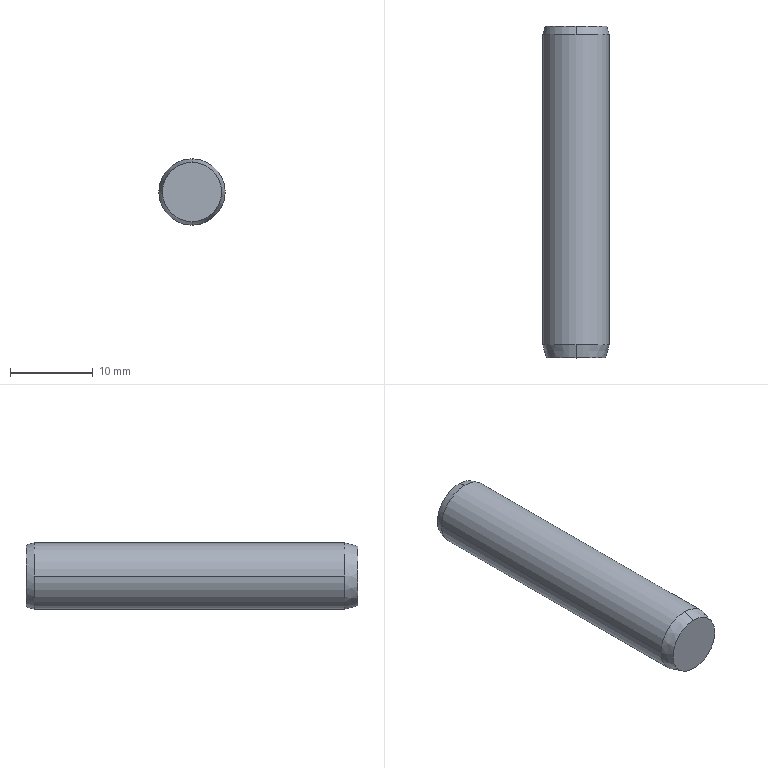Part | STEP file | 1 solid | 16 faces | box 8 x 40 x 8 mm | volume 1821 mm3 | cone 8 | cylinder 6 | plane 2 | commonest cylinder face diameters 4.134 x2 5.3 x2 8 x2
STEP:
#1=CARTESIAN_POINT('',(0.,-40.,3.571));
#2=VERTEX_POINT('',#1);
#3=CARTESIAN_POINT('',(0.,-40.,-3.571));
#4=VERTEX_POINT('',#3);
#5=CARTESIAN_POINT('',(0.,-40.,0.));
#6=DIRECTION('',(0.,1.,0.));
#7=DIRECTION('',(0.,0.,1.));
#8=AXIS2_PLACEMENT_3D('',#5,#6,#7);
#9=CIRCLE('',#8,3.571);
#10=EDGE_CURVE('',#2,#4,#9,.T.);
#11=ORIENTED_EDGE('',*,*,#10,.T.);
#12=CARTESIAN_POINT('',(0.,-38.4,-4.));
#13=VERTEX_POINT('',#12);
#14=CARTESIAN_POINT('',(0.,-40.,-3.571));
#15=DIRECTION('',(0.,0.9659,-0.2588));
#16=VECTOR('',#15,1000.);
#17=LINE('',#14,#16);
#18=EDGE_CURVE('',#4,#13,#17,.T.);
#19=ORIENTED_EDGE('',*,*,#18,.T.);
#20=CARTESIAN_POINT('',(4.,-38.4,0.));
#21=VERTEX_POINT('',#20);
#22=CARTESIAN_POINT('',(0.,-38.4,0.));
#23=DIRECTION('',(0.,1.,0.));
#24=DIRECTION('',(0.,0.,1.));
#25=AXIS2_PLACEMENT_3D('',#22,#23,#24);
#26=CIRCLE('',#25,4.);
#27=EDGE_CURVE('',#21,#13,#26,.T.);
#28=ORIENTED_EDGE('',*,*,#27,.F.);
#29=CARTESIAN_POINT('',(0.,-38.4,4.));
#30=VERTEX_POINT('',#29);
#31=CARTESIAN_POINT('',(0.,-38.4,0.));
#32=DIRECTION('',(0.,1.,0.));
#33=DIRECTION('',(0.,0.,1.));
#34=AXIS2_PLACEMENT_3D('',#31,#32,#33);
#35=CIRCLE('',#34,4.);
#36=EDGE_CURVE('',#30,#21,#35,.T.);
#37=ORIENTED_EDGE('',*,*,#36,.F.);
#38=CARTESIAN_POINT('',(0.,-40.,3.571));
#39=DIRECTION('',(0.,0.9659,0.2588));
#40=VECTOR('',#39,1000.);
#41=LINE('',#38,#40);
#42=EDGE_CURVE('',#2,#30,#41,.T.);
#43=ORIENTED_EDGE('',*,*,#42,.F.);
#44=EDGE_LOOP('',(#11,#19,#28,#37,#43));
#45=FACE_OUTER_BOUND('',#44,.T.);
#46=CARTESIAN_POINT('',(0.,-40.,0.));
#47=DIRECTION('',(0.,1.,0.));
#48=DIRECTION('',(0.,0.,1.));
#49=AXIS2_PLACEMENT_3D('',#46,#47,#48);
#50=CONICAL_SURFACE('',#49,3.571,0.2618);
#51=ADVANCED_FACE('',(#45),#50,.T.);
#52=CARTESIAN_POINT('',(-4.,-38.4,0.));
#53=VERTEX_POINT('',#52);
#54=CARTESIAN_POINT('',(0.,-38.4,0.));
#55=DIRECTION('',(0.,1.,0.));
#56=DIRECTION('',(0.,0.,1.));
#57=AXIS2_PLACEMENT_3D('',#54,#55,#56);
#58=CIRCLE('',#57,4.);
#59=EDGE_CURVE('',#53,#30,#58,.T.);
#60=ORIENTED_EDGE('',*,*,#59,.T.);
#61=ORIENTED_EDGE('',*,*,#36,.T.);
#62=CARTESIAN_POINT('',(4.,-1.,0.));
#63=VERTEX_POINT('',#62);
#64=CARTESIAN_POINT('',(4.,-13.193,0.));
#65=DIRECTION('',(0.,1.,0.));
#66=VECTOR('',#65,1000.);
#67=LINE('',#64,#66);
#68=EDGE_CURVE('',#21,#63,#67,.T.);
#69=ORIENTED_EDGE('',*,*,#68,.T.);
#70=CARTESIAN_POINT('',(0.,-1.,4.));
#71=VERTEX_POINT('',#70);
#72=CARTESIAN_POINT('',(0.,-1.,0.));
#73=DIRECTION('',(0.,1.,0.));
#74=DIRECTION('',(0.,0.,1.));
#75=AXIS2_PLACEMENT_3D('',#72,#73,#74);
#76=CIRCLE('',#75,4.);
#77=EDGE_CURVE('',#71,#63,#76,.T.);
#78=ORIENTED_EDGE('',*,*,#77,.F.);
#79=CARTESIAN_POINT('',(-4.,-1.,0.));
#80=VERTEX_POINT('',#79);
#81=CARTESIAN_POINT('',(0.,-1.,0.));
#82=DIRECTION('',(0.,1.,0.));
#83=DIRECTION('',(0.,0.,1.));
#84=AXIS2_PLACEMENT_3D('',#81,#82,#83);
#85=CIRCLE('',#84,4.);
#86=EDGE_CURVE('',#80,#71,#85,.T.);
#87=ORIENTED_EDGE('',*,*,#86,.F.);
#88=CARTESIAN_POINT('',(-4.,-13.193,0.));
#89=DIRECTION('',(0.,1.,0.));
#90=VECTOR('',#89,1000.);
#91=LINE('',#88,#90);
#92=EDGE_CURVE('',#53,#80,#91,.T.);
#93=ORIENTED_EDGE('',*,*,#92,.F.);
#94=EDGE_LOOP('',(#60,#61,#69,#78,#87,#93));
#95=FACE_OUTER_BOUND('',#94,.T.);
#96=CARTESIAN_POINT('',(0.,-13.193,0.));
#97=DIRECTION('',(0.,1.,0.));
#98=DIRECTION('',(-1.,0.,0.));
#99=AXIS2_PLACEMENT_3D('',#96,#97,#98);
#100=CYLINDRICAL_SURFACE('',#99,4.);
#101=ADVANCED_FACE('',(#95),#100,.T.);
#102=CARTESIAN_POINT('',(0.,0.,3.732));
#103=VERTEX_POINT('',#102);
#104=CARTESIAN_POINT('',(0.,0.,-3.732));
#105=VERTEX_POINT('',#104);
#106=CARTESIAN_POINT('',(0.,0.,0.));
#107=DIRECTION('',(0.,1.,0.));
#108=DIRECTION('',(0.,0.,1.));
#109=AXIS2_PLACEMENT_3D('',#106,#107,#108);
#110=CIRCLE('',#109,3.732);
#111=EDGE_CURVE('',#103,#105,#110,.T.);
#112=ORIENTED_EDGE('',*,*,#111,.F.);
#113=CARTESIAN_POINT('',(0.,-1.,4.));
#114=DIRECTION('',(0.,-0.9659,0.2588));
#115=VECTOR('',#114,1000.);
#116=LINE('',#113,#115);
#117=EDGE_CURVE('',#103,#71,#116,.T.);
#118=ORIENTED_EDGE('',*,*,#117,.T.);
#119=ORIENTED_EDGE('',*,*,#77,.T.);
#120=CARTESIAN_POINT('',(0.,-1.,-4.));
#121=VERTEX_POINT('',#120);
#122=CARTESIAN_POINT('',(0.,-1.,0.));
#123=DIRECTION('',(0.,1.,0.));
#124=DIRECTION('',(0.,0.,1.));
#125=AXIS2_PLACEMENT_3D('',#122,#123,#124);
#126=CIRCLE('',#125,4.);
#127=EDGE_CURVE('',#63,#121,#126,.T.);
#128=ORIENTED_EDGE('',*,*,#127,.T.);
#129=CARTESIAN_POINT('',(0.,-1.,-4.));
#130=DIRECTION('',(0.,-0.9659,-0.2588));
#131=VECTOR('',#130,1000.);
#132=LINE('',#129,#131);
#133=EDGE_CURVE('',#105,#121,#132,.T.);
#134=ORIENTED_EDGE('',*,*,#133,.F.);
#135=EDGE_LOOP('',(#112,#118,#119,#128,#134));
#136=FACE_OUTER_BOUND('',#135,.T.);
#137=CARTESIAN_POINT('',(0.,-1.,0.));
#138=DIRECTION('',(0.,-1.,0.));
#139=DIRECTION('',(0.,0.,-1.));
#140=AXIS2_PLACEMENT_3D('',#137,#138,#139);
#141=CONICAL_SURFACE('',#140,4.,0.2618);
#142=ADVANCED_FACE('',(#136),#141,.T.);
#143=CARTESIAN_POINT('',(0.,-13.193,0.));
#144=VERTEX_POINT('',#143);
#145=CARTESIAN_POINT('',(-2.067,-12.,0.));
#146=VERTEX_POINT('',#145);
#147=CARTESIAN_POINT('',(-2.067,-12.,0.));
#148=DIRECTION('',(-0.866,0.5,0.));
#149=VECTOR('',#148,1000.);
#150=LINE('',#147,#149);
#151=EDGE_CURVE('',#144,#146,#150,.T.);
#152=ORIENTED_EDGE('',*,*,#151,.F.);
#153=CARTESIAN_POINT('',(2.067,-12.,0.));
#154=VERTEX_POINT('',#153);
#155=CARTESIAN_POINT('',(2.067,-12.,0.));
#156=DIRECTION('',(0.866,0.5,0.));
#157=VECTOR('',#156,1000.);
#158=LINE('',#155,#157);
#159=EDGE_CURVE('',#144,#154,#158,.T.);
#160=ORIENTED_EDGE('',*,*,#159,.T.);
#161=CARTESIAN_POINT('',(0.,-12.,0.));
#162=DIRECTION('',(0.,1.,0.));
#163=DIRECTION('',(-1.,0.,0.));
#164=AXIS2_PLACEMENT_3D('',#161,#162,#163);
#165=CIRCLE('',#164,2.067);
#166=EDGE_CURVE('',#154,#146,#165,.T.);
#167=ORIENTED_EDGE('',*,*,#166,.T.);
#168=EDGE_LOOP('',(#152,#160,#167));
#169=FACE_OUTER_BOUND('',#168,.T.);
#170=CARTESIAN_POINT('',(0.,-12.,0.));
#171=DIRECTION('',(0.,1.,0.));
#172=DIRECTION('',(-1.,0.,0.));
#173=AXIS2_PLACEMENT_3D('',#170,#171,#172);
#174=CONICAL_SURFACE('',#173,2.067,1.047);
#175=ADVANCED_FACE('',(#169),#174,.F.);
#176=ORIENTED_EDGE('',*,*,#166,.F.);
#177=CARTESIAN_POINT('',(2.067,-1.537,0.));
#178=VERTEX_POINT('',#177);
#179=CARTESIAN_POINT('',(2.067,-13.193,0.));
#180=DIRECTION('',(0.,1.,0.));
#181=VECTOR('',#180,1000.);
#182=LINE('',#179,#181);
#183=EDGE_CURVE('',#154,#178,#182,.T.);
#184=ORIENTED_EDGE('',*,*,#183,.T.);
#185=CARTESIAN_POINT('',(-2.067,-1.537,0.));
#186=VERTEX_POINT('',#185);
#187=CARTESIAN_POINT('',(0.,-1.537,0.));
#188=DIRECTION('',(0.,1.,0.));
#189=DIRECTION('',(-1.,0.,0.));
#190=AXIS2_PLACEMENT_3D('',#187,#188,#189);
#191=CIRCLE('',#190,2.067);
#192=EDGE_CURVE('',#178,#186,#191,.T.);
#193=ORIENTED_EDGE('',*,*,#192,.T.);
#194=CARTESIAN_POINT('',(-2.067,-13.193,0.));
#195=DIRECTION('',(0.,1.,0.));
#196=VECTOR('',#195,1000.);
#197=LINE('',#194,#196);
#198=EDGE_CURVE('',#146,#186,#197,.T.);
#199=ORIENTED_EDGE('',*,*,#198,.F.);
#200=EDGE_LOOP('',(#176,#184,#193,#199));
#201=FACE_OUTER_BOUND('',#200,.T.);
#202=CARTESIAN_POINT('',(0.,-13.193,0.));
#203=DIRECTION('',(0.,1.,0.));
#204=DIRECTION('',(-1.,0.,0.));
#205=AXIS2_PLACEMENT_3D('',#202,#203,#204);
#206=CYLINDRICAL_SURFACE('',#205,2.067);
#207=ADVANCED_FACE('',(#201),#206,.F.);
#208=ORIENTED_EDGE('',*,*,#192,.F.);
#209=CARTESIAN_POINT('',(2.65,-1.2,0.));
#210=VERTEX_POINT('',#209);
#211=CARTESIAN_POINT('',(2.65,-1.2,0.));
#212=DIRECTION('',(0.866,0.5,0.));
#213=VECTOR('',#212,1000.);
#214=LINE('',#211,#213);
#215=EDGE_CURVE('',#178,#210,#214,.T.);
#216=ORIENTED_EDGE('',*,*,#215,.T.);
#217=CARTESIAN_POINT('',(-2.65,-1.2,0.));
#218=VERTEX_POINT('',#217);
#219=CARTESIAN_POINT('',(0.,-1.2,0.));
#220=DIRECTION('',(0.,1.,0.));
#221=DIRECTION('',(-1.,0.,0.));
#222=AXIS2_PLACEMENT_3D('',#219,#220,#221);
#223=CIRCLE('',#222,2.65);
#224=EDGE_CURVE('',#210,#218,#223,.T.);
#225=ORIENTED_EDGE('',*,*,#224,.T.);
#226=CARTESIAN_POINT('',(-2.65,-1.2,0.));
#227=DIRECTION('',(-0.866,0.5,0.));
#228=VECTOR('',#227,1000.);
#229=LINE('',#226,#228);
#230=EDGE_CURVE('',#186,#218,#229,.T.);
#231=ORIENTED_EDGE('',*,*,#230,.F.);
#232=EDGE_LOOP('',(#208,#216,#225,#231));
#233=FACE_OUTER_BOUND('',#232,.T.);
#234=CARTESIAN_POINT('',(0.,-1.2,0.));
#235=DIRECTION('',(0.,1.,0.));
#236=DIRECTION('',(-1.,0.,0.));
#237=AXIS2_PLACEMENT_3D('',#234,#235,#236);
#238=CONICAL_SURFACE('',#237,2.65,1.047);
#239=ADVANCED_FACE('',(#233),#238,.F.);
#240=ORIENTED_EDGE('',*,*,#224,.F.);
#241=CARTESIAN_POINT('',(2.65,0.,0.));
#242=VERTEX_POINT('',#241);
#243=CARTESIAN_POINT('',(2.65,-13.193,0.));
#244=DIRECTION('',(0.,1.,0.));
#245=VECTOR('',#244,1000.);
#246=LINE('',#243,#245);
#247=EDGE_CURVE('',#210,#242,#246,.T.);
#248=ORIENTED_EDGE('',*,*,#247,.T.);
#249=CARTESIAN_POINT('',(-2.65,0.,0.));
#250=VERTEX_POINT('',#249);
#251=CARTESIAN_POINT('',(0.,0.,0.));
#252=DIRECTION('',(0.,1.,0.));
#253=DIRECTION('',(-1.,0.,0.));
#254=AXIS2_PLACEMENT_3D('',#251,#252,#253);
#255=CIRCLE('',#254,2.65);
#256=EDGE_CURVE('',#242,#250,#255,.T.);
#257=ORIENTED_EDGE('',*,*,#256,.T.);
#258=CARTESIAN_POINT('',(-2.65,-13.193,0.));
#259=DIRECTION('',(0.,1.,0.));
#260=VECTOR('',#259,1000.);
#261=LINE('',#258,#260);
#262=EDGE_CURVE('',#218,#250,#261,.T.);
#263=ORIENTED_EDGE('',*,*,#262,.F.);
#264=EDGE_LOOP('',(#240,#248,#257,#263));
#265=FACE_OUTER_BOUND('',#264,.T.);
#266=CARTESIAN_POINT('',(0.,-13.193,0.));
#267=DIRECTION('',(0.,1.,0.));
#268=DIRECTION('',(-1.,0.,0.));
#269=AXIS2_PLACEMENT_3D('',#266,#267,#268);
#270=CYLINDRICAL_SURFACE('',#269,2.65);
#271=ADVANCED_FACE('',(#265),#270,.F.);
#272=CARTESIAN_POINT('',(0.,0.,0.));
#273=DIRECTION('',(0.,1.,0.));
#274=DIRECTION('',(-1.,0.,0.));
#275=AXIS2_PLACEMENT_3D('',#272,#273,#274);
#276=CIRCLE('',#275,2.65);
#277=EDGE_CURVE('',#250,#242,#276,.T.);
#278=ORIENTED_EDGE('',*,*,#277,.F.);
#279=ORIENTED_EDGE('',*,*,#256,.F.);
#280=EDGE_LOOP('',(#278,#279));
#281=FACE_BOUND('',#280,.T.);
#282=CARTESIAN_POINT('',(0.,0.,0.));
#283=DIRECTION('',(0.,1.,0.));
#284=DIRECTION('',(0.,0.,1.));
#285=AXIS2_PLACEMENT_3D('',#282,#283,#284);
#286=CIRCLE('',#285,3.732);
#287=EDGE_CURVE('',#105,#103,#286,.T.);
#288=ORIENTED_EDGE('',*,*,#287,.T.);
#289=ORIENTED_EDGE('',*,*,#111,.T.);
#290=EDGE_LOOP('',(#288,#289));
#291=FACE_OUTER_BOUND('',#290,.T.);
#292=CARTESIAN_POINT('',(4.,0.,0.));
#293=DIRECTION('',(0.,-1.,0.));
#294=DIRECTION('',(1.,0.,0.));
#295=AXIS2_PLACEMENT_3D('',#292,#293,#294);
#296=PLANE('',#295);
#297=ADVANCED_FACE('',(#281,#291),#296,.F.);
#298=ORIENTED_EDGE('',*,*,#247,.F.);
#299=CARTESIAN_POINT('',(0.,-1.2,0.));
#300=DIRECTION('',(0.,1.,0.));
#301=DIRECTION('',(-1.,0.,0.));
#302=AXIS2_PLACEMENT_3D('',#299,#300,#301);
#303=CIRCLE('',#302,2.65);
#304=EDGE_CURVE('',#218,#210,#303,.T.);
#305=ORIENTED_EDGE('',*,*,#304,.F.);
#306=ORIENTED_EDGE('',*,*,#262,.T.);
#307=ORIENTED_EDGE('',*,*,#277,.T.);
#308=EDGE_LOOP('',(#298,#305,#306,#307));
#309=FACE_OUTER_BOUND('',#308,.T.);
#310=CARTESIAN_POINT('',(0.,-13.193,0.));
#311=DIRECTION('',(0.,1.,0.));
#312=DIRECTION('',(-1.,0.,0.));
#313=AXIS2_PLACEMENT_3D('',#310,#311,#312);
#314=CYLINDRICAL_SURFACE('',#313,2.65);
#315=ADVANCED_FACE('',(#309),#314,.F.);
#316=ORIENTED_EDGE('',*,*,#215,.F.);
#317=CARTESIAN_POINT('',(0.,-1.537,0.));
#318=DIRECTION('',(0.,1.,0.));
#319=DIRECTION('',(-1.,0.,0.));
#320=AXIS2_PLACEMENT_3D('',#317,#318,#319);
#321=CIRCLE('',#320,2.067);
#322=EDGE_CURVE('',#186,#178,#321,.T.);
#323=ORIENTED_EDGE('',*,*,#322,.F.);
#324=ORIENTED_EDGE('',*,*,#230,.T.);
#325=ORIENTED_EDGE('',*,*,#304,.T.);
#326=EDGE_LOOP('',(#316,#323,#324,#325));
#327=FACE_OUTER_BOUND('',#326,.T.);
#328=CARTESIAN_POINT('',(0.,-1.2,0.));
#329=DIRECTION('',(0.,1.,0.));
#330=DIRECTION('',(-1.,0.,0.));
#331=AXIS2_PLACEMENT_3D('',#328,#329,#330);
#332=CONICAL_SURFACE('',#331,2.65,1.047);
#333=ADVANCED_FACE('',(#327),#332,.F.);
#334=ORIENTED_EDGE('',*,*,#183,.F.);
#335=CARTESIAN_POINT('',(0.,-12.,0.));
#336=DIRECTION('',(0.,1.,0.));
#337=DIRECTION('',(-1.,0.,0.));
#338=AXIS2_PLACEMENT_3D('',#335,#336,#337);
#339=CIRCLE('',#338,2.067);
#340=EDGE_CURVE('',#146,#154,#339,.T.);
#341=ORIENTED_EDGE('',*,*,#340,.F.);
#342=ORIENTED_EDGE('',*,*,#198,.T.);
#343=ORIENTED_EDGE('',*,*,#322,.T.);
#344=EDGE_LOOP('',(#334,#341,#342,#343));
#345=FACE_OUTER_BOUND('',#344,.T.);
#346=CARTESIAN_POINT('',(0.,-13.193,0.));
#347=DIRECTION('',(0.,1.,0.));
#348=DIRECTION('',(-1.,0.,0.));
#349=AXIS2_PLACEMENT_3D('',#346,#347,#348);
#350=CYLINDRICAL_SURFACE('',#349,2.067);
#351=ADVANCED_FACE('',(#345),#350,.F.);
#352=ORIENTED_EDGE('',*,*,#159,.F.);
#353=ORIENTED_EDGE('',*,*,#151,.T.);
#354=ORIENTED_EDGE('',*,*,#340,.T.);
#355=EDGE_LOOP('',(#352,#353,#354));
#356=FACE_OUTER_BOUND('',#355,.T.);
#357=CARTESIAN_POINT('',(0.,-12.,0.));
#358=DIRECTION('',(0.,1.,0.));
#359=DIRECTION('',(-1.,0.,0.));
#360=AXIS2_PLACEMENT_3D('',#357,#358,#359);
#361=CONICAL_SURFACE('',#360,2.067,1.047);
#362=ADVANCED_FACE('',(#356),#361,.F.);
#363=ORIENTED_EDGE('',*,*,#117,.F.);
#364=ORIENTED_EDGE('',*,*,#287,.F.);
#365=ORIENTED_EDGE('',*,*,#133,.T.);
#366=CARTESIAN_POINT('',(0.,-1.,0.));
#367=DIRECTION('',(0.,1.,0.));
#368=DIRECTION('',(0.,0.,1.));
#369=AXIS2_PLACEMENT_3D('',#366,#367,#368);
#370=CIRCLE('',#369,4.);
#371=EDGE_CURVE('',#121,#80,#370,.T.);
#372=ORIENTED_EDGE('',*,*,#371,.T.);
#373=ORIENTED_EDGE('',*,*,#86,.T.);
#374=EDGE_LOOP('',(#363,#364,#365,#372,#373));
#375=FACE_OUTER_BOUND('',#374,.T.);
#376=CARTESIAN_POINT('',(0.,-1.,0.));
#377=DIRECTION('',(0.,-1.,0.));
#378=DIRECTION('',(0.,0.,-1.));
#379=AXIS2_PLACEMENT_3D('',#376,#377,#378);
#380=CONICAL_SURFACE('',#379,4.,0.2618);
#381=ADVANCED_FACE('',(#375),#380,.T.);
#382=ORIENTED_EDGE('',*,*,#68,.F.);
#383=ORIENTED_EDGE('',*,*,#27,.T.);
#384=CARTESIAN_POINT('',(0.,-38.4,0.));
#385=DIRECTION('',(0.,1.,0.));
#386=DIRECTION('',(0.,0.,1.));
#387=AXIS2_PLACEMENT_3D('',#384,#385,#386);
#388=CIRCLE('',#387,4.);
#389=EDGE_CURVE('',#13,#53,#388,.T.);
#390=ORIENTED_EDGE('',*,*,#389,.T.);
#391=ORIENTED_EDGE('',*,*,#92,.T.);
#392=ORIENTED_EDGE('',*,*,#371,.F.);
#393=ORIENTED_EDGE('',*,*,#127,.F.);
#394=EDGE_LOOP('',(#382,#383,#390,#391,#392,#393));
#395=FACE_OUTER_BOUND('',#394,.T.);
#396=CARTESIAN_POINT('',(0.,-13.193,0.));
#397=DIRECTION('',(0.,1.,0.));
#398=DIRECTION('',(-1.,0.,0.));
#399=AXIS2_PLACEMENT_3D('',#396,#397,#398);
#400=CYLINDRICAL_SURFACE('',#399,4.);
#401=ADVANCED_FACE('',(#395),#400,.T.);
#402=ORIENTED_EDGE('',*,*,#18,.F.);
#403=CARTESIAN_POINT('',(0.,-40.,0.));
#404=DIRECTION('',(0.,1.,0.));
#405=DIRECTION('',(0.,0.,1.));
#406=AXIS2_PLACEMENT_3D('',#403,#404,#405);
#407=CIRCLE('',#406,3.571);
#408=EDGE_CURVE('',#4,#2,#407,.T.);
#409=ORIENTED_EDGE('',*,*,#408,.T.);
#410=ORIENTED_EDGE('',*,*,#42,.T.);
#411=ORIENTED_EDGE('',*,*,#59,.F.);
#412=ORIENTED_EDGE('',*,*,#389,.F.);
#413=EDGE_LOOP('',(#402,#409,#410,#411,#412));
#414=FACE_OUTER_BOUND('',#413,.T.);
#415=CARTESIAN_POINT('',(0.,-40.,0.));
#416=DIRECTION('',(0.,1.,0.));
#417=DIRECTION('',(0.,0.,1.));
#418=AXIS2_PLACEMENT_3D('',#415,#416,#417);
#419=CONICAL_SURFACE('',#418,3.571,0.2618);
#420=ADVANCED_FACE('',(#414),#419,.T.);
#421=ORIENTED_EDGE('',*,*,#10,.F.);
#422=ORIENTED_EDGE('',*,*,#408,.F.);
#423=EDGE_LOOP('',(#421,#422));
#424=FACE_OUTER_BOUND('',#423,.T.);
#425=CARTESIAN_POINT('',(0.,-40.,0.));
#426=DIRECTION('',(0.,1.,0.));
#427=DIRECTION('',(-1.,0.,0.));
#428=AXIS2_PLACEMENT_3D('',#425,#426,#427);
#429=PLANE('',#428);
#430=ADVANCED_FACE('',(#424),#429,.F.);
#431=CLOSED_SHELL('',(#51,#101,#142,#175,#207,#239,#271,#297,#315,#333,#351,#362,#381,#401,#420,#430));
#432=MANIFOLD_SOLID_BREP('',#431);
#433=CARTESIAN_POINT('',(0.,0.,0.));
#434=DIRECTION('',(0.,0.,1.));
#435=DIRECTION('',(1.,0.,0.));
#436=AXIS2_PLACEMENT_3D('',#433,#434,#435);
#437=(LENGTH_UNIT()NAMED_UNIT(*)SI_UNIT(.MILLI.,.METRE.));
#438=UNCERTAINTY_MEASURE_WITH_UNIT(LENGTH_MEASURE(0.00001),#437,'','');
#439=(NAMED_UNIT(*)PLANE_ANGLE_UNIT()SI_UNIT($,.RADIAN.));
#440=(NAMED_UNIT(*)SI_UNIT($,.STERADIAN.)SOLID_ANGLE_UNIT());
#441=(GEOMETRIC_REPRESENTATION_CONTEXT(3)GLOBAL_UNCERTAINTY_ASSIGNED_CONTEXT((#438))GLOBAL_UNIT_ASSIGNED_CONTEXT((#437,#439,#440))REPRESENTATION_CONTEXT('',''));
#442=ADVANCED_BREP_SHAPE_REPRESENTATION('',(#432,#436),#441);